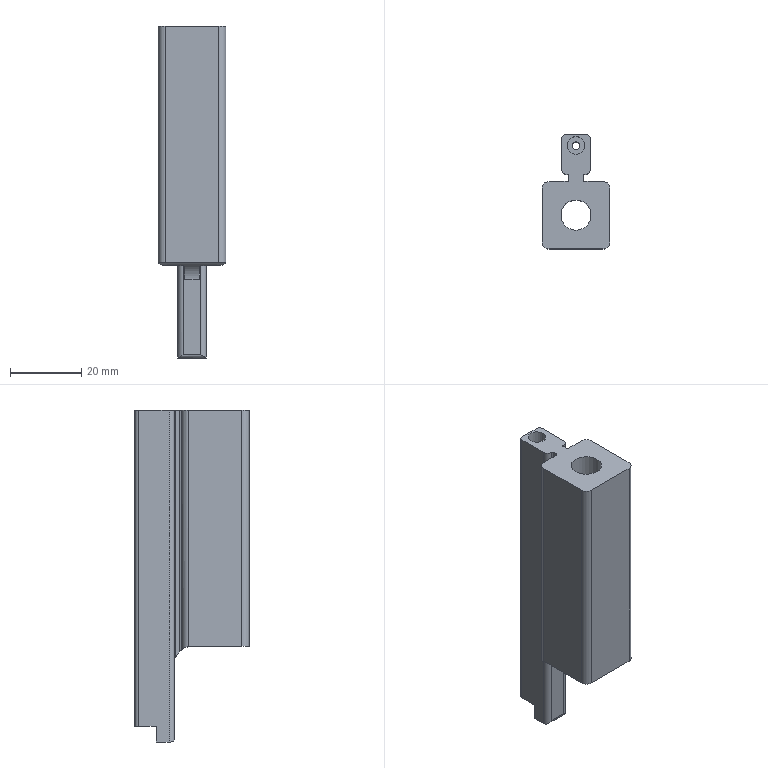Part | NX | features PU-3 2 | 1 solid | 36 faces | box 19 x 32.15 x 93.5 mm | volume 23137 mm3 | plane 18 | cylinder 18 | commonest cylinder face diameters 4 x4 2 x3 0.6 x2 1 x2 3 x2 2.101 x1
STEP:
#1=CARTESIAN_POINT('',(2391.569,-949.525,919.216));
#2=VERTEX_POINT('',#1);
#3=CARTESIAN_POINT('',(2391.569,-945.272,919.216));
#4=DIRECTION('',(0.,0.,1.));
#5=DIRECTION('',(0.,-1.,0.));
#6=AXIS2_PLACEMENT_3D('',#3,#4,#5);
#7=CIRCLE('',#6,4.253);
#8=EDGE_CURVE('',#2,#2,#7,.T.);
#9=ORIENTED_EDGE('',*,*,#8,.T.);
#10=EDGE_LOOP('',(#9));
#11=FACE_BOUND('',#10,.T.);
#12=CARTESIAN_POINT('',(2391.569,-952.522,919.216));
#13=VERTEX_POINT('',#12);
#14=CARTESIAN_POINT('',(2391.569,-945.272,919.216));
#15=DIRECTION('',(0.,0.,-1.));
#16=DIRECTION('',(0.,-1.,0.));
#17=AXIS2_PLACEMENT_3D('',#14,#15,#16);
#18=CIRCLE('',#17,7.25);
#19=EDGE_CURVE('',#13,#13,#18,.T.);
#20=ORIENTED_EDGE('',*,*,#19,.T.);
#21=EDGE_LOOP('',(#20));
#22=FACE_BOUND('',#21,.T.);
#23=CARTESIAN_POINT('',(2449.49,-1418.303,919.216));
#24=DIRECTION('',(0.,0.,1.));
#25=DIRECTION('',(0.,1.,0.));
#26=AXIS2_PLACEMENT_3D('',#23,#24,#25);
#27=PLANE('',#26);
#28=ADVANCED_FACE('',(#11,#22),#27,.F.);
#29=CARTESIAN_POINT('',(2394.78,-938.772,879.217));
#30=VERTEX_POINT('',#29);
#31=CARTESIAN_POINT('',(2388.357,-938.772,879.217));
#32=VERTEX_POINT('',#31);
#33=CARTESIAN_POINT('',(2394.78,-938.772,879.217));
#34=CARTESIAN_POINT('',(2393.777,-938.276,879.217));
#35=CARTESIAN_POINT('',(2391.576,-937.768,879.103));
#36=CARTESIAN_POINT('',(2389.361,-938.276,879.217));
#37=CARTESIAN_POINT('',(2388.357,-938.772,879.217));
#38=B_SPLINE_CURVE_WITH_KNOTS('',3,(#33,#34,#35,#36,#37),.UNSPECIFIED.,.F.,.F.,(4,1,4),(0.,0.003304,0.006609),.UNSPECIFIED.);
#39=EDGE_CURVE('',#30,#32,#38,.T.);
#40=ORIENTED_EDGE('',*,*,#39,.F.);
#41=CARTESIAN_POINT('',(2391.569,-945.272,879.217));
#42=DIRECTION('',(0.,0.,1.));
#43=DIRECTION('',(0.,1.,0.));
#44=AXIS2_PLACEMENT_3D('',#41,#42,#43);
#45=CIRCLE('',#44,7.25);
#46=EDGE_CURVE('',#32,#30,#45,.T.);
#47=ORIENTED_EDGE('',*,*,#46,.F.);
#48=EDGE_LOOP('',(#40,#47));
#49=FACE_BOUND('',#48,.T.);
#50=ORIENTED_EDGE('',*,*,#19,.F.);
#51=EDGE_LOOP('',(#50));
#52=FACE_BOUND('',#51,.T.);
#53=CARTESIAN_POINT('',(2391.569,-945.272,912.216));
#54=DIRECTION('',(0.,0.,-1.));
#55=DIRECTION('',(0.,-1.,0.));
#56=AXIS2_PLACEMENT_3D('',#53,#54,#55);
#57=CYLINDRICAL_SURFACE('',#56,7.25);
#58=ADVANCED_FACE('',(#49,#52),#57,.F.);
#59=CARTESIAN_POINT('',(2382.069,-952.772,879.217));
#60=VERTEX_POINT('',#59);
#61=CARTESIAN_POINT('',(2382.069,-938.772,879.217));
#62=VERTEX_POINT('',#61);
#63=CARTESIAN_POINT('',(2382.069,-1068.421,879.217));
#64=DIRECTION('',(0.,1.,0.));
#65=VECTOR('',#64,1000.);
#66=LINE('',#63,#65);
#67=EDGE_CURVE('',#60,#62,#66,.T.);
#68=ORIENTED_EDGE('',*,*,#67,.T.);
#69=CARTESIAN_POINT('',(3137.566,-938.772,879.217));
#70=DIRECTION('',(1.,0.,0.));
#71=VECTOR('',#70,1000.);
#72=LINE('',#69,#71);
#73=EDGE_CURVE('',#62,#32,#72,.T.);
#74=ORIENTED_EDGE('',*,*,#73,.T.);
#75=ORIENTED_EDGE('',*,*,#46,.T.);
#76=CARTESIAN_POINT('',(2401.069,-938.772,879.217));
#77=VERTEX_POINT('',#76);
#78=CARTESIAN_POINT('',(3137.566,-938.772,879.217));
#79=DIRECTION('',(1.,0.,0.));
#80=VECTOR('',#79,1000.);
#81=LINE('',#78,#80);
#82=EDGE_CURVE('',#30,#77,#81,.T.);
#83=ORIENTED_EDGE('',*,*,#82,.T.);
#84=CARTESIAN_POINT('',(2401.069,-952.772,879.217));
#85=VERTEX_POINT('',#84);
#86=CARTESIAN_POINT('',(2401.069,-1068.421,879.217));
#87=DIRECTION('',(0.,-1.,0.));
#88=VECTOR('',#87,1000.);
#89=LINE('',#86,#88);
#90=EDGE_CURVE('',#77,#85,#89,.T.);
#91=ORIENTED_EDGE('',*,*,#90,.T.);
#92=CARTESIAN_POINT('',(2399.069,-954.772,879.217));
#93=VERTEX_POINT('',#92);
#94=CARTESIAN_POINT('',(2399.069,-952.772,879.217));
#95=DIRECTION('',(0.,0.,-1.));
#96=DIRECTION('',(0.,1.,0.));
#97=AXIS2_PLACEMENT_3D('',#94,#95,#96);
#98=CIRCLE('',#97,2.);
#99=EDGE_CURVE('',#85,#93,#98,.T.);
#100=ORIENTED_EDGE('',*,*,#99,.T.);
#101=CARTESIAN_POINT('',(2384.069,-954.772,879.217));
#102=VERTEX_POINT('',#101);
#103=CARTESIAN_POINT('',(3137.566,-954.772,879.217));
#104=DIRECTION('',(-1.,0.,0.));
#105=VECTOR('',#104,1000.);
#106=LINE('',#103,#105);
#107=EDGE_CURVE('',#93,#102,#106,.T.);
#108=ORIENTED_EDGE('',*,*,#107,.T.);
#109=CARTESIAN_POINT('',(2384.069,-952.772,879.217));
#110=DIRECTION('',(0.,0.,-1.));
#111=DIRECTION('',(0.,1.,0.));
#112=AXIS2_PLACEMENT_3D('',#109,#110,#111);
#113=CIRCLE('',#112,2.);
#114=EDGE_CURVE('',#102,#60,#113,.T.);
#115=ORIENTED_EDGE('',*,*,#114,.T.);
#116=EDGE_LOOP('',(#68,#74,#75,#83,#91,#100,#108,#115));
#117=FACE_BOUND('',#116,.T.);
#118=CARTESIAN_POINT('',(3137.566,-1068.421,879.217));
#119=DIRECTION('',(0.,0.,-1.));
#120=DIRECTION('',(1.,0.,0.));
#121=AXIS2_PLACEMENT_3D('',#118,#119,#120);
#122=PLANE('',#121);
#123=ADVANCED_FACE('',(#117),#122,.T.);
#124=CARTESIAN_POINT('',(2391.569,-941.019,945.716));
#125=VERTEX_POINT('',#124);
#126=CARTESIAN_POINT('',(2391.569,-945.272,945.716));
#127=DIRECTION('',(0.,0.,-1.));
#128=DIRECTION('',(0.,1.,0.));
#129=AXIS2_PLACEMENT_3D('',#126,#127,#128);
#130=CIRCLE('',#129,4.253);
#131=EDGE_CURVE('',#125,#125,#130,.F.);
#132=ORIENTED_EDGE('',*,*,#131,.T.);
#133=EDGE_LOOP('',(#132));
#134=FACE_BOUND('',#133,.T.);
#135=ORIENTED_EDGE('',*,*,#8,.F.);
#136=EDGE_LOOP('',(#135));
#137=FACE_BOUND('',#136,.T.);
#138=CARTESIAN_POINT('',(2391.569,-945.272,947.216));
#139=DIRECTION('',(0.,0.,-1.));
#140=DIRECTION('',(0.,-1.,0.));
#141=AXIS2_PLACEMENT_3D('',#138,#139,#140);
#142=CYLINDRICAL_SURFACE('',#141,4.253);
#143=ADVANCED_FACE('',(#134,#137),#142,.F.);
#144=CARTESIAN_POINT('',(2393.569,-935.272,877.787));
#145=VERTEX_POINT('',#144);
#146=CARTESIAN_POINT('',(2393.569,-934.072,875.922));
#147=VERTEX_POINT('',#146);
#148=CARTESIAN_POINT('',(2393.569,-938.772,874.217));
#149=DIRECTION('',(-1.,0.,0.));
#150=DIRECTION('',(0.,0.,-1.));
#151=AXIS2_PLACEMENT_3D('',#148,#149,#150);
#152=CIRCLE('',#151,5.);
#153=EDGE_CURVE('',#145,#147,#152,.T.);
#154=ORIENTED_EDGE('',*,*,#153,.T.);
#155=CARTESIAN_POINT('',(2393.569,-934.072,945.716));
#156=VERTEX_POINT('',#155);
#157=CARTESIAN_POINT('',(2393.569,-934.072,945.716));
#158=DIRECTION('',(0.,0.,-1.));
#159=VECTOR('',#158,1000.);
#160=LINE('',#157,#159);
#161=EDGE_CURVE('',#147,#156,#160,.F.);
#162=ORIENTED_EDGE('',*,*,#161,.T.);
#163=CARTESIAN_POINT('',(2393.569,-935.272,945.716));
#164=VERTEX_POINT('',#163);
#165=CARTESIAN_POINT('',(2393.569,-933.722,945.716));
#166=DIRECTION('',(0.,-1.,0.));
#167=VECTOR('',#166,1000.);
#168=LINE('',#165,#167);
#169=EDGE_CURVE('',#156,#164,#168,.T.);
#170=ORIENTED_EDGE('',*,*,#169,.T.);
#171=CARTESIAN_POINT('',(2393.569,-935.272,929.216));
#172=DIRECTION('',(0.,0.,1.));
#173=VECTOR('',#172,1000.);
#174=LINE('',#171,#173);
#175=EDGE_CURVE('',#145,#164,#174,.T.);
#176=ORIENTED_EDGE('',*,*,#175,.F.);
#177=EDGE_LOOP('',(#154,#162,#170,#176));
#178=FACE_BOUND('',#177,.T.);
#179=CARTESIAN_POINT('',(2393.569,-933.722,929.216));
#180=DIRECTION('',(-1.,0.,0.));
#181=DIRECTION('',(0.,0.,-1.));
#182=AXIS2_PLACEMENT_3D('',#179,#180,#181);
#183=PLANE('',#182);
#184=ADVANCED_FACE('',(#178),#183,.F.);
#185=CARTESIAN_POINT('',(2394.069,-935.772,878.217));
#186=VERTEX_POINT('',#185);
#187=CARTESIAN_POINT('',(2394.069,-935.772,878.217));
#188=CARTESIAN_POINT('',(2393.759,-935.772,878.217));
#189=CARTESIAN_POINT('',(2393.569,-935.492,878.003));
#190=CARTESIAN_POINT('',(2393.569,-935.272,877.787));
#191=B_SPLINE_CURVE_WITH_KNOTS('',3,(#187,#188,#189,#190),.UNSPECIFIED.,.F.,.F.,(4,4),(0.,0.0009149),.UNSPECIFIED.);
#192=EDGE_CURVE('',#186,#145,#191,.T.);
#193=ORIENTED_EDGE('',*,*,#192,.T.);
#194=ORIENTED_EDGE('',*,*,#175,.T.);
#195=CARTESIAN_POINT('',(2394.069,-935.772,945.716));
#196=VERTEX_POINT('',#195);
#197=CARTESIAN_POINT('',(2394.069,-935.272,945.716));
#198=DIRECTION('',(0.,0.,-1.));
#199=DIRECTION('',(-1.,0.,0.));
#200=AXIS2_PLACEMENT_3D('',#197,#198,#199);
#201=CIRCLE('',#200,0.5);
#202=EDGE_CURVE('',#164,#196,#201,.F.);
#203=ORIENTED_EDGE('',*,*,#202,.T.);
#204=CARTESIAN_POINT('',(2394.069,-935.772,916.216));
#205=DIRECTION('',(0.,0.,1.));
#206=VECTOR('',#205,1000.);
#207=LINE('',#204,#206);
#208=EDGE_CURVE('',#196,#186,#207,.F.);
#209=ORIENTED_EDGE('',*,*,#208,.T.);
#210=EDGE_LOOP('',(#193,#194,#203,#209));
#211=FACE_BOUND('',#210,.T.);
#212=CARTESIAN_POINT('',(2394.069,-935.272,929.216));
#213=DIRECTION('',(0.,0.,1.));
#214=DIRECTION('',(-1.,0.,0.));
#215=AXIS2_PLACEMENT_3D('',#212,#213,#214);
#216=CYLINDRICAL_SURFACE('',#215,0.5);
#217=ADVANCED_FACE('',(#211),#216,.F.);
#218=CARTESIAN_POINT('',(2399.069,-935.772,945.716));
#219=VERTEX_POINT('',#218);
#220=CARTESIAN_POINT('',(2475.144,-935.772,945.716));
#221=DIRECTION('',(1.,0.,0.));
#222=VECTOR('',#221,1000.);
#223=LINE('',#220,#222);
#224=EDGE_CURVE('',#196,#219,#223,.T.);
#225=ORIENTED_EDGE('',*,*,#224,.T.);
#226=CARTESIAN_POINT('',(2399.069,-935.772,878.217));
#227=VERTEX_POINT('',#226);
#228=CARTESIAN_POINT('',(2399.069,-935.772,945.716));
#229=DIRECTION('',(0.,0.,1.));
#230=VECTOR('',#229,1000.);
#231=LINE('',#228,#230);
#232=EDGE_CURVE('',#227,#219,#231,.T.);
#233=ORIENTED_EDGE('',*,*,#232,.F.);
#234=CARTESIAN_POINT('',(2399.069,-935.772,878.217));
#235=DIRECTION('',(-1.,0.,0.));
#236=VECTOR('',#235,1000.);
#237=LINE('',#234,#236);
#238=EDGE_CURVE('',#227,#186,#237,.T.);
#239=ORIENTED_EDGE('',*,*,#238,.T.);
#240=ORIENTED_EDGE('',*,*,#208,.F.);
#241=EDGE_LOOP('',(#225,#233,#239,#240));
#242=FACE_BOUND('',#241,.T.);
#243=CARTESIAN_POINT('',(2389.319,-935.772,916.216));
#244=DIRECTION('',(0.,1.,0.));
#245=DIRECTION('',(0.,0.,-1.));
#246=AXIS2_PLACEMENT_3D('',#243,#244,#245);
#247=PLANE('',#246);
#248=ADVANCED_FACE('',(#242),#247,.T.);
#249=CARTESIAN_POINT('',(2401.069,-937.772,879.116));
#250=VERTEX_POINT('',#249);
#251=CARTESIAN_POINT('',(2401.069,-937.772,879.116));
#252=CARTESIAN_POINT('',(2401.069,-936.69,878.895));
#253=CARTESIAN_POINT('',(2400.175,-935.772,878.217));
#254=CARTESIAN_POINT('',(2399.069,-935.772,878.217));
#255=B_SPLINE_CURVE_WITH_KNOTS('',3,(#251,#252,#253,#254),.UNSPECIFIED.,.F.,.F.,(4,4),(0.,0.003263),.UNSPECIFIED.);
#256=EDGE_CURVE('',#250,#227,#255,.T.);
#257=ORIENTED_EDGE('',*,*,#256,.T.);
#258=ORIENTED_EDGE('',*,*,#232,.T.);
#259=CARTESIAN_POINT('',(2401.069,-937.772,945.716));
#260=VERTEX_POINT('',#259);
#261=CARTESIAN_POINT('',(2399.069,-937.772,945.716));
#262=DIRECTION('',(0.,0.,-1.));
#263=DIRECTION('',(-1.,0.,0.));
#264=AXIS2_PLACEMENT_3D('',#261,#262,#263);
#265=CIRCLE('',#264,2.);
#266=EDGE_CURVE('',#219,#260,#265,.T.);
#267=ORIENTED_EDGE('',*,*,#266,.T.);
#268=CARTESIAN_POINT('',(2401.069,-937.772,893.217));
#269=DIRECTION('',(0.,0.,1.));
#270=VECTOR('',#269,1000.);
#271=LINE('',#268,#270);
#272=EDGE_CURVE('',#260,#250,#271,.F.);
#273=ORIENTED_EDGE('',*,*,#272,.T.);
#274=EDGE_LOOP('',(#257,#258,#267,#273));
#275=FACE_BOUND('',#274,.T.);
#276=CARTESIAN_POINT('',(2399.069,-937.772,916.216));
#277=DIRECTION('',(0.,0.,-1.));
#278=DIRECTION('',(1.,0.,0.));
#279=AXIS2_PLACEMENT_3D('',#276,#277,#278);
#280=CYLINDRICAL_SURFACE('',#279,2.);
#281=ADVANCED_FACE('',(#275),#280,.T.);
#282=CARTESIAN_POINT('',(2401.069,-952.772,945.716));
#283=VERTEX_POINT('',#282);
#284=CARTESIAN_POINT('',(2401.069,-933.722,945.716));
#285=DIRECTION('',(0.,-1.,0.));
#286=VECTOR('',#285,1000.);
#287=LINE('',#284,#286);
#288=EDGE_CURVE('',#260,#283,#287,.T.);
#289=ORIENTED_EDGE('',*,*,#288,.T.);
#290=CARTESIAN_POINT('',(2401.069,-952.772,929.216));
#291=DIRECTION('',(0.,0.,-1.));
#292=VECTOR('',#291,1000.);
#293=LINE('',#290,#292);
#294=EDGE_CURVE('',#283,#85,#293,.T.);
#295=ORIENTED_EDGE('',*,*,#294,.T.);
#296=ORIENTED_EDGE('',*,*,#90,.F.);
#297=CARTESIAN_POINT('',(2401.069,-938.772,874.217));
#298=DIRECTION('',(-1.,0.,0.));
#299=DIRECTION('',(0.,0.,-1.));
#300=AXIS2_PLACEMENT_3D('',#297,#298,#299);
#301=CIRCLE('',#300,5.);
#302=EDGE_CURVE('',#77,#250,#301,.T.);
#303=ORIENTED_EDGE('',*,*,#302,.T.);
#304=ORIENTED_EDGE('',*,*,#272,.F.);
#305=EDGE_LOOP('',(#289,#295,#296,#303,#304));
#306=FACE_BOUND('',#305,.T.);
#307=CARTESIAN_POINT('',(2401.069,-933.722,929.216));
#308=DIRECTION('',(-1.,0.,0.));
#309=DIRECTION('',(0.,0.,-1.));
#310=AXIS2_PLACEMENT_3D('',#307,#308,#309);
#311=PLANE('',#310);
#312=ADVANCED_FACE('',(#306),#311,.F.);
#313=ORIENTED_EDGE('',*,*,#99,.F.);
#314=ORIENTED_EDGE('',*,*,#294,.F.);
#315=CARTESIAN_POINT('',(2399.069,-954.772,945.716));
#316=VERTEX_POINT('',#315);
#317=CARTESIAN_POINT('',(2399.069,-952.772,945.716));
#318=DIRECTION('',(0.,0.,-1.));
#319=DIRECTION('',(0.,1.,0.));
#320=AXIS2_PLACEMENT_3D('',#317,#318,#319);
#321=CIRCLE('',#320,2.);
#322=EDGE_CURVE('',#316,#283,#321,.F.);
#323=ORIENTED_EDGE('',*,*,#322,.F.);
#324=CARTESIAN_POINT('',(2399.069,-954.772,929.216));
#325=DIRECTION('',(0.,0.,1.));
#326=VECTOR('',#325,1000.);
#327=LINE('',#324,#326);
#328=EDGE_CURVE('',#93,#316,#327,.T.);
#329=ORIENTED_EDGE('',*,*,#328,.F.);
#330=EDGE_LOOP('',(#313,#314,#323,#329));
#331=FACE_BOUND('',#330,.T.);
#332=CARTESIAN_POINT('',(2399.069,-952.772,929.216));
#333=DIRECTION('',(0.,0.,-1.));
#334=DIRECTION('',(0.,-1.,0.));
#335=AXIS2_PLACEMENT_3D('',#332,#333,#334);
#336=CYLINDRICAL_SURFACE('',#335,2.);
#337=ADVANCED_FACE('',(#331),#336,.T.);
#338=CARTESIAN_POINT('',(2384.069,-954.772,945.716));
#339=VERTEX_POINT('',#338);
#340=CARTESIAN_POINT('',(2401.644,-954.772,945.716));
#341=DIRECTION('',(-1.,0.,0.));
#342=VECTOR('',#341,1000.);
#343=LINE('',#340,#342);
#344=EDGE_CURVE('',#316,#339,#343,.T.);
#345=ORIENTED_EDGE('',*,*,#344,.T.);
#346=CARTESIAN_POINT('',(2384.069,-954.772,929.216));
#347=DIRECTION('',(0.,0.,-1.));
#348=VECTOR('',#347,1000.);
#349=LINE('',#346,#348);
#350=EDGE_CURVE('',#339,#102,#349,.T.);
#351=ORIENTED_EDGE('',*,*,#350,.T.);
#352=ORIENTED_EDGE('',*,*,#107,.F.);
#353=ORIENTED_EDGE('',*,*,#328,.T.);
#354=EDGE_LOOP('',(#345,#351,#352,#353));
#355=FACE_BOUND('',#354,.T.);
#356=CARTESIAN_POINT('',(2401.644,-954.772,929.216));
#357=DIRECTION('',(0.,1.,0.));
#358=DIRECTION('',(0.,0.,1.));
#359=AXIS2_PLACEMENT_3D('',#356,#357,#358);
#360=PLANE('',#359);
#361=ADVANCED_FACE('',(#355),#360,.F.);
#362=ORIENTED_EDGE('',*,*,#114,.F.);
#363=ORIENTED_EDGE('',*,*,#350,.F.);
#364=CARTESIAN_POINT('',(2382.069,-952.772,945.716));
#365=VERTEX_POINT('',#364);
#366=CARTESIAN_POINT('',(2384.069,-952.772,945.716));
#367=DIRECTION('',(0.,0.,-1.));
#368=DIRECTION('',(0.,1.,0.));
#369=AXIS2_PLACEMENT_3D('',#366,#367,#368);
#370=CIRCLE('',#369,2.);
#371=EDGE_CURVE('',#365,#339,#370,.F.);
#372=ORIENTED_EDGE('',*,*,#371,.F.);
#373=CARTESIAN_POINT('',(2382.069,-952.772,929.216));
#374=DIRECTION('',(0.,0.,1.));
#375=VECTOR('',#374,1000.);
#376=LINE('',#373,#375);
#377=EDGE_CURVE('',#60,#365,#376,.T.);
#378=ORIENTED_EDGE('',*,*,#377,.F.);
#379=EDGE_LOOP('',(#362,#363,#372,#378));
#380=FACE_BOUND('',#379,.T.);
#381=CARTESIAN_POINT('',(2384.069,-952.772,929.216));
#382=DIRECTION('',(0.,0.,1.));
#383=DIRECTION('',(0.,1.,0.));
#384=AXIS2_PLACEMENT_3D('',#381,#382,#383);
#385=CYLINDRICAL_SURFACE('',#384,2.);
#386=ADVANCED_FACE('',(#380),#385,.T.);
#387=ORIENTED_EDGE('',*,*,#67,.F.);
#388=ORIENTED_EDGE('',*,*,#377,.T.);
#389=CARTESIAN_POINT('',(2382.069,-937.772,945.716));
#390=VERTEX_POINT('',#389);
#391=CARTESIAN_POINT('',(2382.069,-933.772,945.716));
#392=DIRECTION('',(0.,1.,0.));
#393=VECTOR('',#392,1000.);
#394=LINE('',#391,#393);
#395=EDGE_CURVE('',#365,#390,#394,.T.);
#396=ORIENTED_EDGE('',*,*,#395,.T.);
#397=CARTESIAN_POINT('',(2382.069,-937.772,879.116));
#398=VERTEX_POINT('',#397);
#399=CARTESIAN_POINT('',(2382.069,-937.772,929.216));
#400=DIRECTION('',(0.,0.,-1.));
#401=VECTOR('',#400,1000.);
#402=LINE('',#399,#401);
#403=EDGE_CURVE('',#390,#398,#402,.T.);
#404=ORIENTED_EDGE('',*,*,#403,.T.);
#405=CARTESIAN_POINT('',(2382.069,-938.772,874.217));
#406=DIRECTION('',(1.,0.,0.));
#407=DIRECTION('',(0.,0.,1.));
#408=AXIS2_PLACEMENT_3D('',#405,#406,#407);
#409=CIRCLE('',#408,5.);
#410=EDGE_CURVE('',#398,#62,#409,.T.);
#411=ORIENTED_EDGE('',*,*,#410,.T.);
#412=EDGE_LOOP('',(#387,#388,#396,#404,#411));
#413=FACE_BOUND('',#412,.T.);
#414=CARTESIAN_POINT('',(2382.069,-933.772,929.216));
#415=DIRECTION('',(1.,0.,0.));
#416=DIRECTION('',(0.,0.,1.));
#417=AXIS2_PLACEMENT_3D('',#414,#415,#416);
#418=PLANE('',#417);
#419=ADVANCED_FACE('',(#413),#418,.F.);
#420=CARTESIAN_POINT('',(2384.069,-935.772,945.716));
#421=VERTEX_POINT('',#420);
#422=CARTESIAN_POINT('',(2384.069,-937.772,945.716));
#423=DIRECTION('',(0.,0.,-1.));
#424=DIRECTION('',(0.,1.,0.));
#425=AXIS2_PLACEMENT_3D('',#422,#423,#424);
#426=CIRCLE('',#425,2.);
#427=EDGE_CURVE('',#421,#390,#426,.F.);
#428=ORIENTED_EDGE('',*,*,#427,.F.);
#429=CARTESIAN_POINT('',(2384.069,-935.772,878.217));
#430=VERTEX_POINT('',#429);
#431=CARTESIAN_POINT('',(2384.069,-935.772,894.716));
#432=DIRECTION('',(0.,0.,1.));
#433=VECTOR('',#432,1000.);
#434=LINE('',#431,#433);
#435=EDGE_CURVE('',#430,#421,#434,.T.);
#436=ORIENTED_EDGE('',*,*,#435,.F.);
#437=CARTESIAN_POINT('',(2384.069,-935.772,878.217));
#438=CARTESIAN_POINT('',(2382.962,-935.772,878.217));
#439=CARTESIAN_POINT('',(2382.069,-936.689,878.895));
#440=CARTESIAN_POINT('',(2382.069,-937.772,879.116));
#441=B_SPLINE_CURVE_WITH_KNOTS('',3,(#437,#438,#439,#440),.UNSPECIFIED.,.F.,.F.,(4,4),(0.,0.003264),.UNSPECIFIED.);
#442=EDGE_CURVE('',#430,#398,#441,.T.);
#443=ORIENTED_EDGE('',*,*,#442,.T.);
#444=ORIENTED_EDGE('',*,*,#403,.F.);
#445=EDGE_LOOP('',(#428,#436,#443,#444));
#446=FACE_BOUND('',#445,.T.);
#447=CARTESIAN_POINT('',(2384.069,-937.772,929.216));
#448=DIRECTION('',(0.,0.,-1.));
#449=DIRECTION('',(0.,-1.,0.));
#450=AXIS2_PLACEMENT_3D('',#447,#448,#449);
#451=CYLINDRICAL_SURFACE('',#450,2.);
#452=ADVANCED_FACE('',(#446),#451,.T.);
#453=CARTESIAN_POINT('',(2389.069,-935.772,945.716));
#454=VERTEX_POINT('',#453);
#455=CARTESIAN_POINT('',(2389.069,-935.772,878.217));
#456=VERTEX_POINT('',#455);
#457=CARTESIAN_POINT('',(2389.069,-935.772,895.217));
#458=DIRECTION('',(0.,0.,-1.));
#459=VECTOR('',#458,1000.);
#460=LINE('',#457,#459);
#461=EDGE_CURVE('',#454,#456,#460,.T.);
#462=ORIENTED_EDGE('',*,*,#461,.T.);
#463=CARTESIAN_POINT('',(2386.569,-935.772,878.217));
#464=DIRECTION('',(-1.,0.,0.));
#465=VECTOR('',#464,1000.);
#466=LINE('',#463,#465);
#467=EDGE_CURVE('',#456,#430,#466,.T.);
#468=ORIENTED_EDGE('',*,*,#467,.T.);
#469=ORIENTED_EDGE('',*,*,#435,.T.);
#470=CARTESIAN_POINT('',(2475.144,-935.772,945.716));
#471=DIRECTION('',(1.,0.,0.));
#472=VECTOR('',#471,1000.);
#473=LINE('',#470,#472);
#474=EDGE_CURVE('',#421,#454,#473,.T.);
#475=ORIENTED_EDGE('',*,*,#474,.T.);
#476=EDGE_LOOP('',(#462,#468,#469,#475));
#477=FACE_BOUND('',#476,.T.);
#478=CARTESIAN_POINT('',(2389.319,-935.772,916.216));
#479=DIRECTION('',(0.,1.,0.));
#480=DIRECTION('',(0.,0.,-1.));
#481=AXIS2_PLACEMENT_3D('',#478,#479,#480);
#482=PLANE('',#481);
#483=ADVANCED_FACE('',(#477),#482,.T.);
#484=CARTESIAN_POINT('',(2389.569,-935.272,877.787));
#485=VERTEX_POINT('',#484);
#486=CARTESIAN_POINT('',(2389.569,-935.272,945.716));
#487=VERTEX_POINT('',#486);
#488=CARTESIAN_POINT('',(2389.569,-935.272,937.216));
#489=DIRECTION('',(0.,0.,1.));
#490=VECTOR('',#489,1000.);
#491=LINE('',#488,#490);
#492=EDGE_CURVE('',#485,#487,#491,.T.);
#493=ORIENTED_EDGE('',*,*,#492,.F.);
#494=CARTESIAN_POINT('',(2389.569,-935.272,877.787));
#495=CARTESIAN_POINT('',(2389.569,-935.492,878.003));
#496=CARTESIAN_POINT('',(2389.379,-935.772,878.217));
#497=CARTESIAN_POINT('',(2389.069,-935.772,878.217));
#498=B_SPLINE_CURVE_WITH_KNOTS('',3,(#494,#495,#496,#497),.UNSPECIFIED.,.F.,.F.,(4,4),(0.,0.0009137),.UNSPECIFIED.);
#499=EDGE_CURVE('',#485,#456,#498,.T.);
#500=ORIENTED_EDGE('',*,*,#499,.T.);
#501=ORIENTED_EDGE('',*,*,#461,.F.);
#502=CARTESIAN_POINT('',(2389.069,-935.272,945.716));
#503=DIRECTION('',(0.,0.,-1.));
#504=DIRECTION('',(0.,1.,0.));
#505=AXIS2_PLACEMENT_3D('',#502,#503,#504);
#506=CIRCLE('',#505,0.5);
#507=EDGE_CURVE('',#487,#454,#506,.T.);
#508=ORIENTED_EDGE('',*,*,#507,.F.);
#509=EDGE_LOOP('',(#493,#500,#501,#508));
#510=FACE_BOUND('',#509,.T.);
#511=CARTESIAN_POINT('',(2389.069,-935.272,929.216));
#512=DIRECTION('',(0.,0.,-1.));
#513=DIRECTION('',(0.,-1.,0.));
#514=AXIS2_PLACEMENT_3D('',#511,#512,#513);
#515=CYLINDRICAL_SURFACE('',#514,0.5);
#516=ADVANCED_FACE('',(#510),#515,.F.);
#517=CARTESIAN_POINT('',(2389.569,-934.072,945.716));
#518=VERTEX_POINT('',#517);
#519=CARTESIAN_POINT('',(2389.569,-934.772,945.716));
#520=DIRECTION('',(0.,1.,0.));
#521=VECTOR('',#520,1000.);
#522=LINE('',#519,#521);
#523=EDGE_CURVE('',#487,#518,#522,.T.);
#524=ORIENTED_EDGE('',*,*,#523,.T.);
#525=CARTESIAN_POINT('',(2389.569,-934.072,875.922));
#526=VERTEX_POINT('',#525);
#527=CARTESIAN_POINT('',(2389.569,-934.072,874.217));
#528=DIRECTION('',(0.,0.,1.));
#529=VECTOR('',#528,1000.);
#530=LINE('',#527,#529);
#531=EDGE_CURVE('',#518,#526,#530,.F.);
#532=ORIENTED_EDGE('',*,*,#531,.T.);
#533=CARTESIAN_POINT('',(2389.569,-938.772,874.217));
#534=DIRECTION('',(1.,0.,0.));
#535=DIRECTION('',(0.,0.,1.));
#536=AXIS2_PLACEMENT_3D('',#533,#534,#535);
#537=CIRCLE('',#536,5.);
#538=EDGE_CURVE('',#526,#485,#537,.T.);
#539=ORIENTED_EDGE('',*,*,#538,.T.);
#540=ORIENTED_EDGE('',*,*,#492,.T.);
#541=EDGE_LOOP('',(#524,#532,#539,#540));
#542=FACE_BOUND('',#541,.T.);
#543=CARTESIAN_POINT('',(2389.569,-934.772,929.216));
#544=DIRECTION('',(1.,0.,0.));
#545=DIRECTION('',(0.,0.,1.));
#546=AXIS2_PLACEMENT_3D('',#543,#544,#545);
#547=PLANE('',#546);
#548=ADVANCED_FACE('',(#542),#547,.F.);
#549=ORIENTED_EDGE('',*,*,#302,.F.);
#550=ORIENTED_EDGE('',*,*,#82,.F.);
#551=ORIENTED_EDGE('',*,*,#39,.T.);
#552=ORIENTED_EDGE('',*,*,#73,.F.);
#553=ORIENTED_EDGE('',*,*,#410,.F.);
#554=ORIENTED_EDGE('',*,*,#442,.F.);
#555=ORIENTED_EDGE('',*,*,#467,.F.);
#556=ORIENTED_EDGE('',*,*,#499,.F.);
#557=ORIENTED_EDGE('',*,*,#538,.F.);
#558=CARTESIAN_POINT('',(2389.269,-933.772,874.217));
#559=VERTEX_POINT('',#558);
#560=CARTESIAN_POINT('',(2389.569,-934.072,875.922));
#561=CARTESIAN_POINT('',(2389.569,-933.869,875.364));
#562=CARTESIAN_POINT('',(2389.409,-933.772,874.79));
#563=CARTESIAN_POINT('',(2389.269,-933.772,874.217));
#564=B_SPLINE_CURVE_WITH_KNOTS('',3,(#560,#561,#562,#563),.UNSPECIFIED.,.F.,.F.,(4,4),(0.,0.001771),.UNSPECIFIED.);
#565=EDGE_CURVE('',#526,#559,#564,.T.);
#566=ORIENTED_EDGE('',*,*,#565,.T.);
#567=CARTESIAN_POINT('',(2393.869,-933.772,874.217));
#568=VERTEX_POINT('',#567);
#569=CARTESIAN_POINT('',(3137.566,-933.772,874.217));
#570=DIRECTION('',(1.,0.,0.));
#571=VECTOR('',#570,1000.);
#572=LINE('',#569,#571);
#573=EDGE_CURVE('',#568,#559,#572,.F.);
#574=ORIENTED_EDGE('',*,*,#573,.F.);
#575=CARTESIAN_POINT('',(2393.569,-934.072,875.922));
#576=CARTESIAN_POINT('',(2393.569,-933.869,875.364));
#577=CARTESIAN_POINT('',(2393.728,-933.772,874.79));
#578=CARTESIAN_POINT('',(2393.869,-933.772,874.217));
#579=B_SPLINE_CURVE_WITH_KNOTS('',3,(#575,#576,#577,#578),.UNSPECIFIED.,.F.,.F.,(4,4),(0.,0.001771),.UNSPECIFIED.);
#580=EDGE_CURVE('',#568,#147,#579,.F.);
#581=ORIENTED_EDGE('',*,*,#580,.T.);
#582=ORIENTED_EDGE('',*,*,#153,.F.);
#583=ORIENTED_EDGE('',*,*,#192,.F.);
#584=ORIENTED_EDGE('',*,*,#238,.F.);
#585=ORIENTED_EDGE('',*,*,#256,.F.);
#586=EDGE_LOOP('',(#549,#550,#551,#552,#553,#554,#555,#556,#557,#566,#574,#581,#582,#583,#584,#585));
#587=FACE_BOUND('',#586,.T.);
#588=CARTESIAN_POINT('',(3137.566,-938.772,874.217));
#589=DIRECTION('',(-1.,0.,0.));
#590=DIRECTION('',(0.,-1.,0.));
#591=AXIS2_PLACEMENT_3D('',#588,#589,#590);
#592=CYLINDRICAL_SURFACE('',#591,5.);
#593=ADVANCED_FACE('',(#587),#592,.F.);
#594=CARTESIAN_POINT('',(2394.069,-925.622,945.716));
#595=VERTEX_POINT('',#594);
#596=CARTESIAN_POINT('',(2391.569,-925.622,945.716));
#597=DIRECTION('',(0.,0.,1.));
#598=DIRECTION('',(1.,0.,0.));
#599=AXIS2_PLACEMENT_3D('',#596,#597,#598);
#600=CIRCLE('',#599,2.5);
#601=EDGE_CURVE('',#595,#595,#600,.T.);
#602=ORIENTED_EDGE('',*,*,#601,.F.);
#603=EDGE_LOOP('',(#602));
#604=FACE_BOUND('',#603,.T.);
#605=ORIENTED_EDGE('',*,*,#169,.F.);
#606=CARTESIAN_POINT('',(2393.869,-933.772,945.716));
#607=VERTEX_POINT('',#606);
#608=CARTESIAN_POINT('',(2393.869,-934.072,945.716));
#609=DIRECTION('',(0.,0.,1.));
#610=DIRECTION('',(1.,0.,0.));
#611=AXIS2_PLACEMENT_3D('',#608,#609,#610);
#612=CIRCLE('',#611,0.3);
#613=EDGE_CURVE('',#156,#607,#612,.F.);
#614=ORIENTED_EDGE('',*,*,#613,.T.);
#615=CARTESIAN_POINT('',(2394.069,-933.772,945.716));
#616=VERTEX_POINT('',#615);
#617=CARTESIAN_POINT('',(2388.419,-933.772,945.716));
#618=DIRECTION('',(1.,0.,0.));
#619=VECTOR('',#618,1000.);
#620=LINE('',#617,#619);
#621=EDGE_CURVE('',#607,#616,#620,.T.);
#622=ORIENTED_EDGE('',*,*,#621,.T.);
#623=CARTESIAN_POINT('',(2395.569,-932.272,945.716));
#624=VERTEX_POINT('',#623);
#625=CARTESIAN_POINT('',(2394.069,-932.272,945.716));
#626=DIRECTION('',(0.,0.,1.));
#627=DIRECTION('',(1.,0.,0.));
#628=AXIS2_PLACEMENT_3D('',#625,#626,#627);
#629=CIRCLE('',#628,1.5);
#630=EDGE_CURVE('',#616,#624,#629,.T.);
#631=ORIENTED_EDGE('',*,*,#630,.T.);
#632=CARTESIAN_POINT('',(2395.569,-923.622,945.716));
#633=VERTEX_POINT('',#632);
#634=CARTESIAN_POINT('',(2395.569,-932.772,945.716));
#635=DIRECTION('',(0.,1.,0.));
#636=VECTOR('',#635,1000.);
#637=LINE('',#634,#636);
#638=EDGE_CURVE('',#624,#633,#637,.T.);
#639=ORIENTED_EDGE('',*,*,#638,.T.);
#640=CARTESIAN_POINT('',(2394.569,-922.622,945.716));
#641=VERTEX_POINT('',#640);
#642=CARTESIAN_POINT('',(2394.569,-923.622,945.716));
#643=DIRECTION('',(0.,0.,1.));
#644=DIRECTION('',(1.,0.,0.));
#645=AXIS2_PLACEMENT_3D('',#642,#643,#644);
#646=CIRCLE('',#645,1.);
#647=EDGE_CURVE('',#641,#633,#646,.F.);
#648=ORIENTED_EDGE('',*,*,#647,.F.);
#649=CARTESIAN_POINT('',(2388.569,-922.622,945.716));
#650=VERTEX_POINT('',#649);
#651=CARTESIAN_POINT('',(2393.069,-922.622,945.716));
#652=DIRECTION('',(-1.,0.,0.));
#653=VECTOR('',#652,1000.);
#654=LINE('',#651,#653);
#655=EDGE_CURVE('',#641,#650,#654,.T.);
#656=ORIENTED_EDGE('',*,*,#655,.T.);
#657=CARTESIAN_POINT('',(2387.569,-923.622,945.716));
#658=VERTEX_POINT('',#657);
#659=CARTESIAN_POINT('',(2388.569,-923.622,945.716));
#660=DIRECTION('',(0.,0.,1.));
#661=DIRECTION('',(1.,0.,0.));
#662=AXIS2_PLACEMENT_3D('',#659,#660,#661);
#663=CIRCLE('',#662,1.);
#664=EDGE_CURVE('',#658,#650,#663,.F.);
#665=ORIENTED_EDGE('',*,*,#664,.F.);
#666=CARTESIAN_POINT('',(2387.569,-932.272,945.716));
#667=VERTEX_POINT('',#666);
#668=CARTESIAN_POINT('',(2387.569,-925.122,945.716));
#669=DIRECTION('',(0.,-1.,0.));
#670=VECTOR('',#669,1000.);
#671=LINE('',#668,#670);
#672=EDGE_CURVE('',#658,#667,#671,.T.);
#673=ORIENTED_EDGE('',*,*,#672,.T.);
#674=CARTESIAN_POINT('',(2389.069,-933.772,945.716));
#675=VERTEX_POINT('',#674);
#676=CARTESIAN_POINT('',(2389.069,-932.272,945.716));
#677=DIRECTION('',(0.,0.,1.));
#678=DIRECTION('',(1.,0.,0.));
#679=AXIS2_PLACEMENT_3D('',#676,#677,#678);
#680=CIRCLE('',#679,1.5);
#681=EDGE_CURVE('',#667,#675,#680,.T.);
#682=ORIENTED_EDGE('',*,*,#681,.T.);
#683=CARTESIAN_POINT('',(2389.269,-933.772,945.716));
#684=VERTEX_POINT('',#683);
#685=CARTESIAN_POINT('',(2388.419,-933.772,945.716));
#686=DIRECTION('',(1.,0.,0.));
#687=VECTOR('',#686,1000.);
#688=LINE('',#685,#687);
#689=EDGE_CURVE('',#675,#684,#688,.T.);
#690=ORIENTED_EDGE('',*,*,#689,.T.);
#691=CARTESIAN_POINT('',(2389.269,-934.072,945.716));
#692=DIRECTION('',(0.,0.,1.));
#693=DIRECTION('',(1.,0.,0.));
#694=AXIS2_PLACEMENT_3D('',#691,#692,#693);
#695=CIRCLE('',#694,0.3);
#696=EDGE_CURVE('',#684,#518,#695,.F.);
#697=ORIENTED_EDGE('',*,*,#696,.T.);
#698=ORIENTED_EDGE('',*,*,#523,.F.);
#699=ORIENTED_EDGE('',*,*,#507,.T.);
#700=ORIENTED_EDGE('',*,*,#474,.F.);
#701=ORIENTED_EDGE('',*,*,#427,.T.);
#702=ORIENTED_EDGE('',*,*,#395,.F.);
#703=ORIENTED_EDGE('',*,*,#371,.T.);
#704=ORIENTED_EDGE('',*,*,#344,.F.);
#705=ORIENTED_EDGE('',*,*,#322,.T.);
#706=ORIENTED_EDGE('',*,*,#288,.F.);
#707=ORIENTED_EDGE('',*,*,#266,.F.);
#708=ORIENTED_EDGE('',*,*,#224,.F.);
#709=ORIENTED_EDGE('',*,*,#202,.F.);
#710=EDGE_LOOP('',(#605,#614,#622,#631,#639,#648,#656,#665,#673,#682,#690,#697,#698,#699,#700,#701,#702,#703,#704,#705,#706,#707,#708,#709));
#711=FACE_BOUND('',#710,.T.);
#712=ORIENTED_EDGE('',*,*,#131,.F.);
#713=EDGE_LOOP('',(#712));
#714=FACE_BOUND('',#713,.T.);
#715=CARTESIAN_POINT('',(2252.088,-970.272,945.716));
#716=DIRECTION('',(0.,0.,1.));
#717=DIRECTION('',(-1.,0.,0.));
#718=AXIS2_PLACEMENT_3D('',#715,#716,#717);
#719=PLANE('',#718);
#720=ADVANCED_FACE('',(#604,#711,#714),#719,.T.);
#721=ORIENTED_EDGE('',*,*,#621,.F.);
#722=CARTESIAN_POINT('',(2393.869,-933.772,874.217));
#723=DIRECTION('',(0.,0.,-1.));
#724=VECTOR('',#723,1000.);
#725=LINE('',#722,#724);
#726=EDGE_CURVE('',#607,#568,#725,.T.);
#727=ORIENTED_EDGE('',*,*,#726,.T.);
#728=ORIENTED_EDGE('',*,*,#573,.T.);
#729=CARTESIAN_POINT('',(2389.269,-933.772,945.716));
#730=DIRECTION('',(0.,0.,1.));
#731=VECTOR('',#730,1000.);
#732=LINE('',#729,#731);
#733=EDGE_CURVE('',#559,#684,#732,.T.);
#734=ORIENTED_EDGE('',*,*,#733,.T.);
#735=ORIENTED_EDGE('',*,*,#689,.F.);
#736=CARTESIAN_POINT('',(2389.069,-933.772,853.216));
#737=VERTEX_POINT('',#736);
#738=CARTESIAN_POINT('',(2389.069,-933.772,940.716));
#739=DIRECTION('',(0.,0.,-1.));
#740=VECTOR('',#739,1000.);
#741=LINE('',#738,#740);
#742=EDGE_CURVE('',#675,#737,#741,.T.);
#743=ORIENTED_EDGE('',*,*,#742,.T.);
#744=CARTESIAN_POINT('',(2394.069,-933.772,853.216));
#745=VERTEX_POINT('',#744);
#746=CARTESIAN_POINT('',(2388.419,-933.772,853.216));
#747=DIRECTION('',(1.,0.,0.));
#748=VECTOR('',#747,1000.);
#749=LINE('',#746,#748);
#750=EDGE_CURVE('',#737,#745,#749,.T.);
#751=ORIENTED_EDGE('',*,*,#750,.T.);
#752=CARTESIAN_POINT('',(2394.069,-933.772,940.716));
#753=DIRECTION('',(0.,0.,1.));
#754=VECTOR('',#753,1000.);
#755=LINE('',#752,#754);
#756=EDGE_CURVE('',#745,#616,#755,.T.);
#757=ORIENTED_EDGE('',*,*,#756,.T.);
#758=EDGE_LOOP('',(#721,#727,#728,#734,#735,#743,#751,#757));
#759=FACE_BOUND('',#758,.T.);
#760=CARTESIAN_POINT('',(2388.419,-933.772,940.716));
#761=DIRECTION('',(0.,1.,0.));
#762=DIRECTION('',(0.,0.,-1.));
#763=AXIS2_PLACEMENT_3D('',#760,#761,#762);
#764=PLANE('',#763);
#765=ADVANCED_FACE('',(#759),#764,.F.);
#766=ORIENTED_EDGE('',*,*,#750,.F.);
#767=CARTESIAN_POINT('',(2387.655,-932.772,852.216));
#768=VERTEX_POINT('',#767);
#769=CARTESIAN_POINT('',(2389.069,-933.772,853.216));
#770=CARTESIAN_POINT('',(2388.795,-933.772,852.993));
#771=CARTESIAN_POINT('',(2388.242,-933.633,852.541));
#772=CARTESIAN_POINT('',(2387.775,-933.113,852.216));
#773=CARTESIAN_POINT('',(2387.655,-932.772,852.216));
#774=B_SPLINE_CURVE_WITH_KNOTS('',3,(#769,#770,#771,#772,#773),.UNSPECIFIED.,.F.,.F.,(4,1,4),(-0.000007746,0.001052,0.002113),.UNSPECIFIED.);
#775=EDGE_CURVE('',#737,#768,#774,.T.);
#776=ORIENTED_EDGE('',*,*,#775,.T.);
#777=CARTESIAN_POINT('',(2395.483,-932.772,852.216));
#778=VERTEX_POINT('',#777);
#779=CARTESIAN_POINT('',(2260.569,-932.772,852.216));
#780=DIRECTION('',(-1.,0.,0.));
#781=VECTOR('',#780,1000.);
#782=LINE('',#779,#781);
#783=EDGE_CURVE('',#778,#768,#782,.T.);
#784=ORIENTED_EDGE('',*,*,#783,.F.);
#785=CARTESIAN_POINT('',(2395.483,-932.772,852.216));
#786=CARTESIAN_POINT('',(2395.362,-933.113,852.216));
#787=CARTESIAN_POINT('',(2394.896,-933.631,852.541));
#788=CARTESIAN_POINT('',(2394.344,-933.772,852.991));
#789=CARTESIAN_POINT('',(2394.069,-933.772,853.216));
#790=B_SPLINE_CURVE_WITH_KNOTS('',3,(#785,#786,#787,#788,#789),.UNSPECIFIED.,.F.,.F.,(4,1,4),(0.,0.001067,0.002134),.UNSPECIFIED.);
#791=EDGE_CURVE('',#778,#745,#790,.T.);
#792=ORIENTED_EDGE('',*,*,#791,.T.);
#793=EDGE_LOOP('',(#766,#776,#784,#792));
#794=FACE_BOUND('',#793,.T.);
#795=CARTESIAN_POINT('',(2260.569,-932.772,853.216));
#796=DIRECTION('',(-1.,0.,0.));
#797=DIRECTION('',(0.,0.,-1.));
#798=AXIS2_PLACEMENT_3D('',#795,#796,#797);
#799=CYLINDRICAL_SURFACE('',#798,1.);
#800=ADVANCED_FACE('',(#794),#799,.T.);
#801=ORIENTED_EDGE('',*,*,#783,.T.);
#802=CARTESIAN_POINT('',(2387.569,-932.272,852.216));
#803=VERTEX_POINT('',#802);
#804=CARTESIAN_POINT('',(2389.069,-932.272,852.216));
#805=DIRECTION('',(0.,0.,-1.));
#806=DIRECTION('',(-1.,0.,0.));
#807=AXIS2_PLACEMENT_3D('',#804,#805,#806);
#808=CIRCLE('',#807,1.5);
#809=EDGE_CURVE('',#768,#803,#808,.T.);
#810=ORIENTED_EDGE('',*,*,#809,.T.);
#811=CARTESIAN_POINT('',(2387.569,-928.622,852.216));
#812=VERTEX_POINT('',#811);
#813=CARTESIAN_POINT('',(2387.569,-925.122,852.216));
#814=DIRECTION('',(0.,-1.,0.));
#815=VECTOR('',#814,1000.);
#816=LINE('',#813,#815);
#817=EDGE_CURVE('',#812,#803,#816,.T.);
#818=ORIENTED_EDGE('',*,*,#817,.F.);
#819=CARTESIAN_POINT('',(2395.569,-928.622,852.216));
#820=VERTEX_POINT('',#819);
#821=CARTESIAN_POINT('',(2260.569,-928.622,852.216));
#822=DIRECTION('',(-1.,0.,0.));
#823=VECTOR('',#822,1000.);
#824=LINE('',#821,#823);
#825=EDGE_CURVE('',#820,#812,#824,.T.);
#826=ORIENTED_EDGE('',*,*,#825,.F.);
#827=CARTESIAN_POINT('',(2395.569,-932.272,852.216));
#828=VERTEX_POINT('',#827);
#829=CARTESIAN_POINT('',(2395.569,-851.622,852.216));
#830=DIRECTION('',(0.,1.,0.));
#831=VECTOR('',#830,1000.);
#832=LINE('',#829,#831);
#833=EDGE_CURVE('',#828,#820,#832,.T.);
#834=ORIENTED_EDGE('',*,*,#833,.F.);
#835=CARTESIAN_POINT('',(2394.069,-932.272,852.216));
#836=DIRECTION('',(0.,0.,-1.));
#837=DIRECTION('',(-1.,0.,0.));
#838=AXIS2_PLACEMENT_3D('',#835,#836,#837);
#839=CIRCLE('',#838,1.5);
#840=EDGE_CURVE('',#828,#778,#839,.T.);
#841=ORIENTED_EDGE('',*,*,#840,.T.);
#842=EDGE_LOOP('',(#801,#810,#818,#826,#834,#841));
#843=FACE_BOUND('',#842,.T.);
#844=CARTESIAN_POINT('',(2260.569,-851.622,852.216));
#845=DIRECTION('',(0.,0.,1.));
#846=DIRECTION('',(-1.,0.,0.));
#847=AXIS2_PLACEMENT_3D('',#844,#845,#846);
#848=PLANE('',#847);
#849=ADVANCED_FACE('',(#843),#848,.F.);
#850=ORIENTED_EDGE('',*,*,#825,.T.);
#851=CARTESIAN_POINT('',(2387.569,-928.622,856.716));
#852=VERTEX_POINT('',#851);
#853=CARTESIAN_POINT('',(2387.569,-928.622,940.716));
#854=DIRECTION('',(0.,0.,1.));
#855=VECTOR('',#854,1000.);
#856=LINE('',#853,#855);
#857=EDGE_CURVE('',#812,#852,#856,.T.);
#858=ORIENTED_EDGE('',*,*,#857,.T.);
#859=CARTESIAN_POINT('',(2395.569,-928.622,856.716));
#860=VERTEX_POINT('',#859);
#861=CARTESIAN_POINT('',(2260.569,-928.622,856.716));
#862=DIRECTION('',(1.,0.,0.));
#863=VECTOR('',#862,1000.);
#864=LINE('',#861,#863);
#865=EDGE_CURVE('',#852,#860,#864,.T.);
#866=ORIENTED_EDGE('',*,*,#865,.T.);
#867=CARTESIAN_POINT('',(2395.569,-928.622,940.716));
#868=DIRECTION('',(0.,0.,1.));
#869=VECTOR('',#868,1000.);
#870=LINE('',#867,#869);
#871=EDGE_CURVE('',#820,#860,#870,.T.);
#872=ORIENTED_EDGE('',*,*,#871,.F.);
#873=EDGE_LOOP('',(#850,#858,#866,#872));
#874=FACE_BOUND('',#873,.T.);
#875=CARTESIAN_POINT('',(2390.569,-928.622,894.716));
#876=DIRECTION('',(0.,1.,0.));
#877=DIRECTION('',(0.,0.,-1.));
#878=AXIS2_PLACEMENT_3D('',#875,#876,#877);
#879=PLANE('',#878);
#880=ADVANCED_FACE('',(#874),#879,.T.);
#881=CARTESIAN_POINT('',(2392.619,-925.622,856.716));
#882=VERTEX_POINT('',#881);
#883=CARTESIAN_POINT('',(2391.569,-925.622,856.716));
#884=DIRECTION('',(0.,0.,1.));
#885=DIRECTION('',(1.,0.,0.));
#886=AXIS2_PLACEMENT_3D('',#883,#884,#885);
#887=CIRCLE('',#886,1.05);
#888=EDGE_CURVE('',#882,#882,#887,.T.);
#889=ORIENTED_EDGE('',*,*,#888,.T.);
#890=EDGE_LOOP('',(#889));
#891=FACE_BOUND('',#890,.T.);
#892=CARTESIAN_POINT('',(2394.569,-922.622,856.716));
#893=VERTEX_POINT('',#892);
#894=CARTESIAN_POINT('',(2388.569,-922.622,856.716));
#895=VERTEX_POINT('',#894);
#896=CARTESIAN_POINT('',(2260.569,-922.622,856.716));
#897=DIRECTION('',(-1.,0.,0.));
#898=VECTOR('',#897,1000.);
#899=LINE('',#896,#898);
#900=EDGE_CURVE('',#893,#895,#899,.T.);
#901=ORIENTED_EDGE('',*,*,#900,.F.);
#902=CARTESIAN_POINT('',(2395.569,-923.622,856.716));
#903=VERTEX_POINT('',#902);
#904=CARTESIAN_POINT('',(2394.569,-923.622,856.716));
#905=DIRECTION('',(0.,0.,-1.));
#906=DIRECTION('',(-1.,0.,0.));
#907=AXIS2_PLACEMENT_3D('',#904,#905,#906);
#908=CIRCLE('',#907,1.);
#909=EDGE_CURVE('',#903,#893,#908,.F.);
#910=ORIENTED_EDGE('',*,*,#909,.F.);
#911=CARTESIAN_POINT('',(2395.569,-851.622,856.716));
#912=DIRECTION('',(0.,1.,0.));
#913=VECTOR('',#912,1000.);
#914=LINE('',#911,#913);
#915=EDGE_CURVE('',#860,#903,#914,.T.);
#916=ORIENTED_EDGE('',*,*,#915,.F.);
#917=ORIENTED_EDGE('',*,*,#865,.F.);
#918=CARTESIAN_POINT('',(2387.569,-923.622,856.716));
#919=VERTEX_POINT('',#918);
#920=CARTESIAN_POINT('',(2387.569,-851.622,856.716));
#921=DIRECTION('',(0.,-1.,0.));
#922=VECTOR('',#921,1000.);
#923=LINE('',#920,#922);
#924=EDGE_CURVE('',#919,#852,#923,.T.);
#925=ORIENTED_EDGE('',*,*,#924,.F.);
#926=CARTESIAN_POINT('',(2388.569,-923.622,856.716));
#927=DIRECTION('',(0.,0.,-1.));
#928=DIRECTION('',(-1.,0.,0.));
#929=AXIS2_PLACEMENT_3D('',#926,#927,#928);
#930=CIRCLE('',#929,1.);
#931=EDGE_CURVE('',#895,#919,#930,.F.);
#932=ORIENTED_EDGE('',*,*,#931,.F.);
#933=EDGE_LOOP('',(#901,#910,#916,#917,#925,#932));
#934=FACE_BOUND('',#933,.T.);
#935=CARTESIAN_POINT('',(2260.569,-851.622,856.716));
#936=DIRECTION('',(0.,0.,1.));
#937=DIRECTION('',(-1.,0.,0.));
#938=AXIS2_PLACEMENT_3D('',#935,#936,#937);
#939=PLANE('',#938);
#940=ADVANCED_FACE('',(#891,#934),#939,.F.);
#941=ORIENTED_EDGE('',*,*,#664,.T.);
#942=CARTESIAN_POINT('',(2388.569,-922.622,940.716));
#943=DIRECTION('',(0.,0.,-1.));
#944=VECTOR('',#943,1000.);
#945=LINE('',#942,#944);
#946=EDGE_CURVE('',#650,#895,#945,.T.);
#947=ORIENTED_EDGE('',*,*,#946,.T.);
#948=ORIENTED_EDGE('',*,*,#931,.T.);
#949=CARTESIAN_POINT('',(2387.569,-923.622,940.716));
#950=DIRECTION('',(0.,0.,-1.));
#951=VECTOR('',#950,1000.);
#952=LINE('',#949,#951);
#953=EDGE_CURVE('',#919,#658,#952,.F.);
#954=ORIENTED_EDGE('',*,*,#953,.T.);
#955=EDGE_LOOP('',(#941,#947,#948,#954));
#956=FACE_BOUND('',#955,.T.);
#957=CARTESIAN_POINT('',(2388.569,-923.622,940.716));
#958=DIRECTION('',(0.,0.,-1.));
#959=DIRECTION('',(1.,0.,0.));
#960=AXIS2_PLACEMENT_3D('',#957,#958,#959);
#961=CYLINDRICAL_SURFACE('',#960,1.);
#962=ADVANCED_FACE('',(#956),#961,.T.);
#963=ORIENTED_EDGE('',*,*,#655,.F.);
#964=CARTESIAN_POINT('',(2394.569,-922.622,940.716));
#965=DIRECTION('',(0.,0.,-1.));
#966=VECTOR('',#965,1000.);
#967=LINE('',#964,#966);
#968=EDGE_CURVE('',#893,#641,#967,.F.);
#969=ORIENTED_EDGE('',*,*,#968,.F.);
#970=ORIENTED_EDGE('',*,*,#900,.T.);
#971=ORIENTED_EDGE('',*,*,#946,.F.);
#972=EDGE_LOOP('',(#963,#969,#970,#971));
#973=FACE_BOUND('',#972,.T.);
#974=CARTESIAN_POINT('',(2393.069,-922.622,940.716));
#975=DIRECTION('',(0.,-1.,0.));
#976=DIRECTION('',(0.,0.,1.));
#977=AXIS2_PLACEMENT_3D('',#974,#975,#976);
#978=PLANE('',#977);
#979=ADVANCED_FACE('',(#973),#978,.F.);
#980=ORIENTED_EDGE('',*,*,#647,.T.);
#981=CARTESIAN_POINT('',(2395.569,-923.622,940.716));
#982=DIRECTION('',(0.,0.,-1.));
#983=VECTOR('',#982,1000.);
#984=LINE('',#981,#983);
#985=EDGE_CURVE('',#633,#903,#984,.T.);
#986=ORIENTED_EDGE('',*,*,#985,.T.);
#987=ORIENTED_EDGE('',*,*,#909,.T.);
#988=ORIENTED_EDGE('',*,*,#968,.T.);
#989=EDGE_LOOP('',(#980,#986,#987,#988));
#990=FACE_BOUND('',#989,.T.);
#991=CARTESIAN_POINT('',(2394.569,-923.622,940.716));
#992=DIRECTION('',(0.,0.,-1.));
#993=DIRECTION('',(1.,0.,0.));
#994=AXIS2_PLACEMENT_3D('',#991,#992,#993);
#995=CYLINDRICAL_SURFACE('',#994,1.);
#996=ADVANCED_FACE('',(#990),#995,.T.);
#997=ORIENTED_EDGE('',*,*,#985,.F.);
#998=ORIENTED_EDGE('',*,*,#638,.F.);
#999=CARTESIAN_POINT('',(2395.569,-932.272,940.716));
#1000=DIRECTION('',(0.,0.,-1.));
#1001=VECTOR('',#1000,1000.);
#1002=LINE('',#999,#1001);
#1003=EDGE_CURVE('',#624,#828,#1002,.T.);
#1004=ORIENTED_EDGE('',*,*,#1003,.T.);
#1005=ORIENTED_EDGE('',*,*,#833,.T.);
#1006=ORIENTED_EDGE('',*,*,#871,.T.);
#1007=ORIENTED_EDGE('',*,*,#915,.T.);
#1008=EDGE_LOOP('',(#997,#998,#1004,#1005,#1006,#1007));
#1009=FACE_BOUND('',#1008,.T.);
#1010=CARTESIAN_POINT('',(2395.569,-932.772,940.716));
#1011=DIRECTION('',(-1.,0.,0.));
#1012=DIRECTION('',(0.,0.,-1.));
#1013=AXIS2_PLACEMENT_3D('',#1010,#1011,#1012);
#1014=PLANE('',#1013);
#1015=ADVANCED_FACE('',(#1009),#1014,.F.);
#1016=ORIENTED_EDGE('',*,*,#630,.F.);
#1017=ORIENTED_EDGE('',*,*,#756,.F.);
#1018=ORIENTED_EDGE('',*,*,#791,.F.);
#1019=ORIENTED_EDGE('',*,*,#840,.F.);
#1020=ORIENTED_EDGE('',*,*,#1003,.F.);
#1021=EDGE_LOOP('',(#1016,#1017,#1018,#1019,#1020));
#1022=FACE_BOUND('',#1021,.T.);
#1023=CARTESIAN_POINT('',(2394.069,-932.272,940.716));
#1024=DIRECTION('',(0.,0.,-1.));
#1025=DIRECTION('',(1.,0.,0.));
#1026=AXIS2_PLACEMENT_3D('',#1023,#1024,#1025);
#1027=CYLINDRICAL_SURFACE('',#1026,1.5);
#1028=ADVANCED_FACE('',(#1022),#1027,.T.);
#1029=ORIENTED_EDGE('',*,*,#681,.F.);
#1030=CARTESIAN_POINT('',(2387.569,-932.272,940.716));
#1031=DIRECTION('',(0.,0.,1.));
#1032=VECTOR('',#1031,1000.);
#1033=LINE('',#1030,#1032);
#1034=EDGE_CURVE('',#803,#667,#1033,.T.);
#1035=ORIENTED_EDGE('',*,*,#1034,.F.);
#1036=ORIENTED_EDGE('',*,*,#809,.F.);
#1037=ORIENTED_EDGE('',*,*,#775,.F.);
#1038=ORIENTED_EDGE('',*,*,#742,.F.);
#1039=EDGE_LOOP('',(#1029,#1035,#1036,#1037,#1038));
#1040=FACE_BOUND('',#1039,.T.);
#1041=CARTESIAN_POINT('',(2389.069,-932.272,940.716));
#1042=DIRECTION('',(0.,0.,-1.));
#1043=DIRECTION('',(1.,0.,0.));
#1044=AXIS2_PLACEMENT_3D('',#1041,#1042,#1043);
#1045=CYLINDRICAL_SURFACE('',#1044,1.5);
#1046=ADVANCED_FACE('',(#1040),#1045,.T.);
#1047=ORIENTED_EDGE('',*,*,#1034,.T.);
#1048=ORIENTED_EDGE('',*,*,#672,.F.);
#1049=ORIENTED_EDGE('',*,*,#953,.F.);
#1050=ORIENTED_EDGE('',*,*,#924,.T.);
#1051=ORIENTED_EDGE('',*,*,#857,.F.);
#1052=ORIENTED_EDGE('',*,*,#817,.T.);
#1053=EDGE_LOOP('',(#1047,#1048,#1049,#1050,#1051,#1052));
#1054=FACE_BOUND('',#1053,.T.);
#1055=CARTESIAN_POINT('',(2387.569,-925.122,940.716));
#1056=DIRECTION('',(1.,0.,0.));
#1057=DIRECTION('',(0.,0.,1.));
#1058=AXIS2_PLACEMENT_3D('',#1055,#1056,#1057);
#1059=PLANE('',#1058);
#1060=ADVANCED_FACE('',(#1054),#1059,.F.);
#1061=ORIENTED_EDGE('',*,*,#613,.F.);
#1062=ORIENTED_EDGE('',*,*,#161,.F.);
#1063=ORIENTED_EDGE('',*,*,#580,.F.);
#1064=ORIENTED_EDGE('',*,*,#726,.F.);
#1065=EDGE_LOOP('',(#1061,#1062,#1063,#1064));
#1066=FACE_BOUND('',#1065,.T.);
#1067=CARTESIAN_POINT('',(2393.869,-934.072,940.716));
#1068=DIRECTION('',(0.,0.,1.));
#1069=DIRECTION('',(1.,0.,0.));
#1070=AXIS2_PLACEMENT_3D('',#1067,#1068,#1069);
#1071=CYLINDRICAL_SURFACE('',#1070,0.3);
#1072=ADVANCED_FACE('',(#1066),#1071,.F.);
#1073=ORIENTED_EDGE('',*,*,#565,.F.);
#1074=ORIENTED_EDGE('',*,*,#531,.F.);
#1075=ORIENTED_EDGE('',*,*,#696,.F.);
#1076=ORIENTED_EDGE('',*,*,#733,.F.);
#1077=EDGE_LOOP('',(#1073,#1074,#1075,#1076));
#1078=FACE_BOUND('',#1077,.T.);
#1079=CARTESIAN_POINT('',(2389.269,-934.072,940.716));
#1080=DIRECTION('',(0.,0.,-1.));
#1081=DIRECTION('',(-1.,0.,0.));
#1082=AXIS2_PLACEMENT_3D('',#1079,#1080,#1081);
#1083=CYLINDRICAL_SURFACE('',#1082,0.3);
#1084=ADVANCED_FACE('',(#1078),#1083,.F.);
#1085=CARTESIAN_POINT('',(2390.518,-925.622,896.716));
#1086=VERTEX_POINT('',#1085);
#1087=CARTESIAN_POINT('',(2391.569,-925.622,896.716));
#1088=DIRECTION('',(0.,0.,-1.));
#1089=DIRECTION('',(-1.,0.,0.));
#1090=AXIS2_PLACEMENT_3D('',#1087,#1088,#1089);
#1091=CIRCLE('',#1090,1.05);
#1092=EDGE_CURVE('',#1086,#1086,#1091,.T.);
#1093=ORIENTED_EDGE('',*,*,#1092,.F.);
#1094=EDGE_LOOP('',(#1093));
#1095=FACE_BOUND('',#1094,.T.);
#1096=ORIENTED_EDGE('',*,*,#888,.F.);
#1097=EDGE_LOOP('',(#1096));
#1098=FACE_BOUND('',#1097,.T.);
#1099=CARTESIAN_POINT('',(2391.569,-925.622,856.716));
#1100=DIRECTION('',(0.,0.,1.));
#1101=DIRECTION('',(1.,0.,0.));
#1102=AXIS2_PLACEMENT_3D('',#1099,#1100,#1101);
#1103=CYLINDRICAL_SURFACE('',#1102,1.05);
#1104=ADVANCED_FACE('',(#1095,#1098),#1103,.F.);
#1105=ORIENTED_EDGE('',*,*,#1092,.T.);
#1106=EDGE_LOOP('',(#1105));
#1107=FACE_BOUND('',#1106,.T.);
#1108=CARTESIAN_POINT('',(2394.069,-925.622,896.716));
#1109=VERTEX_POINT('',#1108);
#1110=CARTESIAN_POINT('',(2391.569,-925.622,896.716));
#1111=DIRECTION('',(0.,0.,1.));
#1112=DIRECTION('',(1.,0.,0.));
#1113=AXIS2_PLACEMENT_3D('',#1110,#1111,#1112);
#1114=CIRCLE('',#1113,2.5);
#1115=EDGE_CURVE('',#1109,#1109,#1114,.F.);
#1116=ORIENTED_EDGE('',*,*,#1115,.F.);
#1117=EDGE_LOOP('',(#1116));
#1118=FACE_BOUND('',#1117,.T.);
#1119=CARTESIAN_POINT('',(2391.569,-925.622,896.716));
#1120=DIRECTION('',(0.,0.,-1.));
#1121=DIRECTION('',(-1.,0.,0.));
#1122=AXIS2_PLACEMENT_3D('',#1119,#1120,#1121);
#1123=PLANE('',#1122);
#1124=ADVANCED_FACE('',(#1107,#1118),#1123,.F.);
#1125=ORIENTED_EDGE('',*,*,#601,.T.);
#1126=EDGE_LOOP('',(#1125));
#1127=FACE_BOUND('',#1126,.T.);
#1128=ORIENTED_EDGE('',*,*,#1115,.T.);
#1129=EDGE_LOOP('',(#1128));
#1130=FACE_BOUND('',#1129,.T.);
#1131=CARTESIAN_POINT('',(2391.569,-925.622,886.716));
#1132=DIRECTION('',(0.,0.,1.));
#1133=DIRECTION('',(1.,0.,0.));
#1134=AXIS2_PLACEMENT_3D('',#1131,#1132,#1133);
#1135=CYLINDRICAL_SURFACE('',#1134,2.5);
#1136=ADVANCED_FACE('',(#1127,#1130),#1135,.F.);
#1137=CLOSED_SHELL('',(#28,#58,#123,#143,#184,#217,#248,#281,#312,#337,#361,#386,#419,#452,#483,#516,#548,#593,#720,#765,#800,#849,#880,#940,#962,#979,#996,#1015,#1028,#1046,#1060,#1072,#1084,#1104,#1124,#1136));
#1138=MANIFOLD_SOLID_BREP('',#1137);
#1139=(LENGTH_UNIT()NAMED_UNIT(*)SI_UNIT(.MILLI.,.METRE.));
#1140=UNCERTAINTY_MEASURE_WITH_UNIT(LENGTH_MEASURE(0.0508),#1139,'','');
#1141=(NAMED_UNIT(*)PLANE_ANGLE_UNIT()SI_UNIT($,.RADIAN.));
#1142=(NAMED_UNIT(*)SI_UNIT($,.STERADIAN.)SOLID_ANGLE_UNIT());
#1143=(GEOMETRIC_REPRESENTATION_CONTEXT(3)GLOBAL_UNCERTAINTY_ASSIGNED_CONTEXT((#1140))GLOBAL_UNIT_ASSIGNED_CONTEXT((#1139,#1141,#1142))REPRESENTATION_CONTEXT('',''));
#1144=ADVANCED_BREP_SHAPE_REPRESENTATION('',(#1138),#1143);